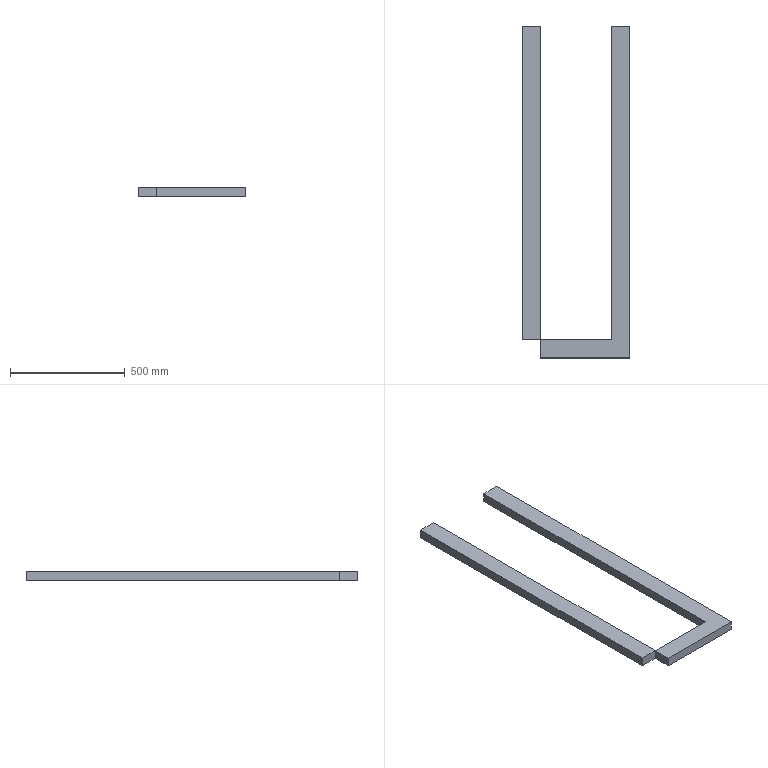Part | STEP file | Connecting profile | 2 solids | 14 faces | box 469.62 x 1446 x 40.945 mm | volume 10095669 mm3 | plane 14
STEP:
#1=CARTESIAN_POINT('',(0.,0.,0.));
#2=DIRECTION('',(0.,0.,1.));
#3=DIRECTION('',(1.,0.,0.));
#4=AXIS2_PLACEMENT_3D('',#1,#2,#3);
#5=CARTESIAN_POINT('',(0.,0.,0.));
#6=VERTEX_POINT('',#5);
#7=CARTESIAN_POINT('',(0.,-80.,0.));
#8=VERTEX_POINT('',#7);
#9=CARTESIAN_POINT('',(0.,-80.,0.));
#10=DIRECTION('',(0.,-1.,0.));
#11=VECTOR('',#10,1.);
#12=LINE('',#9,#11);
#13=CARTESIAN_POINT('',(0.,-80.,40.));
#14=DIRECTION('',(1.,0.,0.));
#15=DIRECTION('',(0.,0.,-1.));
#16=AXIS2_PLACEMENT_3D('',#13,#14,#15);
#17=PLANE('',#16);
#18=CARTESIAN_POINT('',(40.,0.));
#19=DIRECTION('',(0.,-1.));
#20=VECTOR('',#19,1.);
#21=LINE('',#18,#20);
#22=(GEOMETRIC_REPRESENTATION_CONTEXT(2)PARAMETRIC_REPRESENTATION_CONTEXT()REPRESENTATION_CONTEXT('',''));
#23=DEFINITIONAL_REPRESENTATION('',(#21),#22);
#24=PCURVE('',#17,#23);
#25=CARTESIAN_POINT('',(0.,0.,0.));
#26=DIRECTION('',(0.,0.,-1.));
#27=DIRECTION('',(-1.,0.,0.));
#28=AXIS2_PLACEMENT_3D('',#25,#26,#27);
#29=PLANE('',#28);
#30=CARTESIAN_POINT('',(0.,-80.));
#31=DIRECTION('',(0.,-1.));
#32=VECTOR('',#31,1.);
#33=LINE('',#30,#32);
#34=(GEOMETRIC_REPRESENTATION_CONTEXT(2)PARAMETRIC_REPRESENTATION_CONTEXT()REPRESENTATION_CONTEXT('',''));
#35=DEFINITIONAL_REPRESENTATION('',(#33),#34);
#36=PCURVE('',#29,#35);
#37=SURFACE_CURVE('',#12,(#24,#36),.PCURVE_S1.);
#38=EDGE_CURVE('',#6,#8,#37,.T.);
#39=ORIENTED_EDGE('',*,*,#38,.T.);
#40=CARTESIAN_POINT('',(0.,-80.,40.));
#41=VERTEX_POINT('',#40);
#42=CARTESIAN_POINT('',(0.,-80.,40.));
#43=DIRECTION('',(0.,0.,-1.));
#44=VECTOR('',#43,1.);
#45=LINE('',#42,#44);
#46=CARTESIAN_POINT('',(0.,0.));
#47=DIRECTION('',(1.,0.));
#48=VECTOR('',#47,1.);
#49=LINE('',#46,#48);
#50=(GEOMETRIC_REPRESENTATION_CONTEXT(2)PARAMETRIC_REPRESENTATION_CONTEXT()REPRESENTATION_CONTEXT('',''));
#51=DEFINITIONAL_REPRESENTATION('',(#49),#50);
#52=PCURVE('',#17,#51);
#53=CARTESIAN_POINT('',(389.62,-80.,40.));
#54=DIRECTION('',(0.,1.,0.));
#55=DIRECTION('',(-1.,0.,0.));
#56=AXIS2_PLACEMENT_3D('',#53,#54,#55);
#57=PLANE('',#56);
#58=CARTESIAN_POINT('',(389.62,0.));
#59=DIRECTION('',(0.,-1.));
#60=VECTOR('',#59,1.);
#61=LINE('',#58,#60);
#62=(GEOMETRIC_REPRESENTATION_CONTEXT(2)PARAMETRIC_REPRESENTATION_CONTEXT()REPRESENTATION_CONTEXT('',''));
#63=DEFINITIONAL_REPRESENTATION('',(#61),#62);
#64=PCURVE('',#57,#63);
#65=SURFACE_CURVE('',#45,(#52,#64),.PCURVE_S1.);
#66=EDGE_CURVE('',#41,#8,#65,.T.);
#67=ORIENTED_EDGE('',*,*,#66,.F.);
#68=CARTESIAN_POINT('',(0.,0.,40.));
#69=VERTEX_POINT('',#68);
#70=CARTESIAN_POINT('',(0.,-80.,40.));
#71=DIRECTION('',(0.,-1.,0.));
#72=VECTOR('',#71,1.);
#73=LINE('',#70,#72);
#74=CARTESIAN_POINT('',(0.,0.));
#75=DIRECTION('',(0.,-1.));
#76=VECTOR('',#75,1.);
#77=LINE('',#74,#76);
#78=(GEOMETRIC_REPRESENTATION_CONTEXT(2)PARAMETRIC_REPRESENTATION_CONTEXT()REPRESENTATION_CONTEXT('',''));
#79=DEFINITIONAL_REPRESENTATION('',(#77),#78);
#80=PCURVE('',#17,#79);
#81=CARTESIAN_POINT('',(0.,0.,40.));
#82=DIRECTION('',(0.,0.,-1.));
#83=DIRECTION('',(-1.,0.,0.));
#84=AXIS2_PLACEMENT_3D('',#81,#82,#83);
#85=PLANE('',#84);
#86=CARTESIAN_POINT('',(0.,-80.));
#87=DIRECTION('',(0.,-1.));
#88=VECTOR('',#87,1.);
#89=LINE('',#86,#88);
#90=(GEOMETRIC_REPRESENTATION_CONTEXT(2)PARAMETRIC_REPRESENTATION_CONTEXT()REPRESENTATION_CONTEXT('',''));
#91=DEFINITIONAL_REPRESENTATION('',(#89),#90);
#92=PCURVE('',#85,#91);
#93=SURFACE_CURVE('',#73,(#80,#92),.PCURVE_S1.);
#94=EDGE_CURVE('',#69,#41,#93,.T.);
#95=ORIENTED_EDGE('',*,*,#94,.F.);
#96=CARTESIAN_POINT('',(0.,0.,40.));
#97=DIRECTION('',(0.,0.,-1.));
#98=VECTOR('',#97,1.);
#99=LINE('',#96,#98);
#100=CARTESIAN_POINT('',(0.,80.));
#101=DIRECTION('',(1.,0.));
#102=VECTOR('',#101,1.);
#103=LINE('',#100,#102);
#104=(GEOMETRIC_REPRESENTATION_CONTEXT(2)PARAMETRIC_REPRESENTATION_CONTEXT()REPRESENTATION_CONTEXT('',''));
#105=DEFINITIONAL_REPRESENTATION('',(#103),#104);
#106=PCURVE('',#17,#105);
#107=CARTESIAN_POINT('',(0.,0.,40.));
#108=DIRECTION('',(0.,-1.,0.));
#109=DIRECTION('',(0.,0.,-1.));
#110=AXIS2_PLACEMENT_3D('',#107,#108,#109);
#111=PLANE('',#110);
#112=CARTESIAN_POINT('',(0.,0.));
#113=DIRECTION('',(1.,0.));
#114=VECTOR('',#113,1.);
#115=LINE('',#112,#114);
#116=(GEOMETRIC_REPRESENTATION_CONTEXT(2)PARAMETRIC_REPRESENTATION_CONTEXT()REPRESENTATION_CONTEXT('',''));
#117=DEFINITIONAL_REPRESENTATION('',(#115),#116);
#118=PCURVE('',#111,#117);
#119=SURFACE_CURVE('',#99,(#106,#118),.PCURVE_S1.);
#120=EDGE_CURVE('',#69,#6,#119,.T.);
#121=ORIENTED_EDGE('',*,*,#120,.T.);
#122=EDGE_LOOP('',(#39,#67,#95,#121));
#123=FACE_BOUND('',#122,.T.);
#124=ADVANCED_FACE('',(#123),#17,.F.);
#125=CARTESIAN_POINT('',(389.62,-80.,0.));
#126=VERTEX_POINT('',#125);
#127=CARTESIAN_POINT('',(389.62,-80.,0.));
#128=DIRECTION('',(1.,0.,0.));
#129=VECTOR('',#128,1.);
#130=LINE('',#127,#129);
#131=CARTESIAN_POINT('',(0.,-40.));
#132=DIRECTION('',(-1.,0.));
#133=VECTOR('',#132,1.);
#134=LINE('',#131,#133);
#135=(GEOMETRIC_REPRESENTATION_CONTEXT(2)PARAMETRIC_REPRESENTATION_CONTEXT()REPRESENTATION_CONTEXT('',''));
#136=DEFINITIONAL_REPRESENTATION('',(#134),#135);
#137=PCURVE('',#57,#136);
#138=CARTESIAN_POINT('',(-389.62,-80.));
#139=DIRECTION('',(-1.,0.));
#140=VECTOR('',#139,1.);
#141=LINE('',#138,#140);
#142=(GEOMETRIC_REPRESENTATION_CONTEXT(2)PARAMETRIC_REPRESENTATION_CONTEXT()REPRESENTATION_CONTEXT('',''));
#143=DEFINITIONAL_REPRESENTATION('',(#141),#142);
#144=PCURVE('',#29,#143);
#145=SURFACE_CURVE('',#130,(#137,#144),.PCURVE_S1.);
#146=EDGE_CURVE('',#8,#126,#145,.T.);
#147=ORIENTED_EDGE('',*,*,#146,.T.);
#148=CARTESIAN_POINT('',(389.62,-80.,40.));
#149=VERTEX_POINT('',#148);
#150=CARTESIAN_POINT('',(389.62,-80.,40.));
#151=DIRECTION('',(0.,0.,-1.));
#152=VECTOR('',#151,1.);
#153=LINE('',#150,#152);
#154=CARTESIAN_POINT('',(0.,0.));
#155=DIRECTION('',(0.,-1.));
#156=VECTOR('',#155,1.);
#157=LINE('',#154,#156);
#158=(GEOMETRIC_REPRESENTATION_CONTEXT(2)PARAMETRIC_REPRESENTATION_CONTEXT()REPRESENTATION_CONTEXT('',''));
#159=DEFINITIONAL_REPRESENTATION('',(#157),#158);
#160=PCURVE('',#57,#159);
#161=CARTESIAN_POINT('',(389.62,1366.5,40.));
#162=DIRECTION('',(-1.,0.,0.));
#163=DIRECTION('',(0.,-1.,0.));
#164=AXIS2_PLACEMENT_3D('',#161,#162,#163);
#165=PLANE('',#164);
#166=CARTESIAN_POINT('',(1446.5,0.));
#167=DIRECTION('',(0.,-1.));
#168=VECTOR('',#167,1.);
#169=LINE('',#166,#168);
#170=(GEOMETRIC_REPRESENTATION_CONTEXT(2)PARAMETRIC_REPRESENTATION_CONTEXT()REPRESENTATION_CONTEXT('',''));
#171=DEFINITIONAL_REPRESENTATION('',(#169),#170);
#172=PCURVE('',#165,#171);
#173=SURFACE_CURVE('',#153,(#160,#172),.PCURVE_S1.);
#174=EDGE_CURVE('',#149,#126,#173,.T.);
#175=ORIENTED_EDGE('',*,*,#174,.F.);
#176=CARTESIAN_POINT('',(389.62,-80.,40.));
#177=DIRECTION('',(1.,0.,0.));
#178=VECTOR('',#177,1.);
#179=LINE('',#176,#178);
#180=CARTESIAN_POINT('',(0.,0.));
#181=DIRECTION('',(-1.,0.));
#182=VECTOR('',#181,1.);
#183=LINE('',#180,#182);
#184=(GEOMETRIC_REPRESENTATION_CONTEXT(2)PARAMETRIC_REPRESENTATION_CONTEXT()REPRESENTATION_CONTEXT('',''));
#185=DEFINITIONAL_REPRESENTATION('',(#183),#184);
#186=PCURVE('',#57,#185);
#187=CARTESIAN_POINT('',(-389.62,-80.));
#188=DIRECTION('',(-1.,0.));
#189=VECTOR('',#188,1.);
#190=LINE('',#187,#189);
#191=(GEOMETRIC_REPRESENTATION_CONTEXT(2)PARAMETRIC_REPRESENTATION_CONTEXT()REPRESENTATION_CONTEXT('',''));
#192=DEFINITIONAL_REPRESENTATION('',(#190),#191);
#193=PCURVE('',#85,#192);
#194=SURFACE_CURVE('',#179,(#186,#193),.PCURVE_S1.);
#195=EDGE_CURVE('',#41,#149,#194,.T.);
#196=ORIENTED_EDGE('',*,*,#195,.F.);
#197=ORIENTED_EDGE('',*,*,#66,.T.);
#198=EDGE_LOOP('',(#147,#175,#196,#197));
#199=FACE_BOUND('',#198,.T.);
#200=ADVANCED_FACE('',(#199),#57,.F.);
#201=CARTESIAN_POINT('',(389.62,1366.5,0.));
#202=VERTEX_POINT('',#201);
#203=CARTESIAN_POINT('',(389.62,1366.5,0.));
#204=DIRECTION('',(0.,1.,0.));
#205=VECTOR('',#204,1.);
#206=LINE('',#203,#205);
#207=CARTESIAN_POINT('',(0.,-40.));
#208=DIRECTION('',(-1.,0.));
#209=VECTOR('',#208,1.);
#210=LINE('',#207,#209);
#211=(GEOMETRIC_REPRESENTATION_CONTEXT(2)PARAMETRIC_REPRESENTATION_CONTEXT()REPRESENTATION_CONTEXT('',''));
#212=DEFINITIONAL_REPRESENTATION('',(#210),#211);
#213=PCURVE('',#165,#212);
#214=CARTESIAN_POINT('',(-389.62,1366.5));
#215=DIRECTION('',(0.,1.));
#216=VECTOR('',#215,1.);
#217=LINE('',#214,#216);
#218=(GEOMETRIC_REPRESENTATION_CONTEXT(2)PARAMETRIC_REPRESENTATION_CONTEXT()REPRESENTATION_CONTEXT('',''));
#219=DEFINITIONAL_REPRESENTATION('',(#217),#218);
#220=PCURVE('',#29,#219);
#221=SURFACE_CURVE('',#206,(#213,#220),.PCURVE_S1.);
#222=EDGE_CURVE('',#126,#202,#221,.T.);
#223=ORIENTED_EDGE('',*,*,#222,.T.);
#224=CARTESIAN_POINT('',(389.62,1366.5,40.));
#225=VERTEX_POINT('',#224);
#226=CARTESIAN_POINT('',(389.62,1366.5,40.));
#227=DIRECTION('',(0.,0.,-1.));
#228=VECTOR('',#227,1.);
#229=LINE('',#226,#228);
#230=CARTESIAN_POINT('',(0.,0.));
#231=DIRECTION('',(0.,-1.));
#232=VECTOR('',#231,1.);
#233=LINE('',#230,#232);
#234=(GEOMETRIC_REPRESENTATION_CONTEXT(2)PARAMETRIC_REPRESENTATION_CONTEXT()REPRESENTATION_CONTEXT('',''));
#235=DEFINITIONAL_REPRESENTATION('',(#233),#234);
#236=PCURVE('',#165,#235);
#237=CARTESIAN_POINT('',(309.62,1366.5,40.));
#238=DIRECTION('',(0.,-1.,0.));
#239=DIRECTION('',(0.,0.,-1.));
#240=AXIS2_PLACEMENT_3D('',#237,#238,#239);
#241=PLANE('',#240);
#242=CARTESIAN_POINT('',(0.,80.));
#243=DIRECTION('',(1.,0.));
#244=VECTOR('',#243,1.);
#245=LINE('',#242,#244);
#246=(GEOMETRIC_REPRESENTATION_CONTEXT(2)PARAMETRIC_REPRESENTATION_CONTEXT()REPRESENTATION_CONTEXT('',''));
#247=DEFINITIONAL_REPRESENTATION('',(#245),#246);
#248=PCURVE('',#241,#247);
#249=SURFACE_CURVE('',#229,(#236,#248),.PCURVE_S1.);
#250=EDGE_CURVE('',#225,#202,#249,.T.);
#251=ORIENTED_EDGE('',*,*,#250,.F.);
#252=CARTESIAN_POINT('',(389.62,1366.5,40.));
#253=DIRECTION('',(0.,1.,0.));
#254=VECTOR('',#253,1.);
#255=LINE('',#252,#254);
#256=CARTESIAN_POINT('',(0.,0.));
#257=DIRECTION('',(-1.,0.));
#258=VECTOR('',#257,1.);
#259=LINE('',#256,#258);
#260=(GEOMETRIC_REPRESENTATION_CONTEXT(2)PARAMETRIC_REPRESENTATION_CONTEXT()REPRESENTATION_CONTEXT('',''));
#261=DEFINITIONAL_REPRESENTATION('',(#259),#260);
#262=PCURVE('',#165,#261);
#263=CARTESIAN_POINT('',(-389.62,1366.5));
#264=DIRECTION('',(0.,1.));
#265=VECTOR('',#264,1.);
#266=LINE('',#263,#265);
#267=(GEOMETRIC_REPRESENTATION_CONTEXT(2)PARAMETRIC_REPRESENTATION_CONTEXT()REPRESENTATION_CONTEXT('',''));
#268=DEFINITIONAL_REPRESENTATION('',(#266),#267);
#269=PCURVE('',#85,#268);
#270=SURFACE_CURVE('',#255,(#262,#269),.PCURVE_S1.);
#271=EDGE_CURVE('',#149,#225,#270,.T.);
#272=ORIENTED_EDGE('',*,*,#271,.F.);
#273=ORIENTED_EDGE('',*,*,#174,.T.);
#274=EDGE_LOOP('',(#223,#251,#272,#273));
#275=FACE_BOUND('',#274,.T.);
#276=ADVANCED_FACE('',(#275),#165,.F.);
#277=CARTESIAN_POINT('',(309.62,1366.5,0.));
#278=VERTEX_POINT('',#277);
#279=CARTESIAN_POINT('',(309.62,1366.5,0.));
#280=DIRECTION('',(-1.,0.,0.));
#281=VECTOR('',#280,1.);
#282=LINE('',#279,#281);
#283=CARTESIAN_POINT('',(40.,0.));
#284=DIRECTION('',(0.,-1.));
#285=VECTOR('',#284,1.);
#286=LINE('',#283,#285);
#287=(GEOMETRIC_REPRESENTATION_CONTEXT(2)PARAMETRIC_REPRESENTATION_CONTEXT()REPRESENTATION_CONTEXT('',''));
#288=DEFINITIONAL_REPRESENTATION('',(#286),#287);
#289=PCURVE('',#241,#288);
#290=CARTESIAN_POINT('',(-309.62,1366.5));
#291=DIRECTION('',(1.,0.));
#292=VECTOR('',#291,1.);
#293=LINE('',#290,#292);
#294=(GEOMETRIC_REPRESENTATION_CONTEXT(2)PARAMETRIC_REPRESENTATION_CONTEXT()REPRESENTATION_CONTEXT('',''));
#295=DEFINITIONAL_REPRESENTATION('',(#293),#294);
#296=PCURVE('',#29,#295);
#297=SURFACE_CURVE('',#282,(#289,#296),.PCURVE_S1.);
#298=EDGE_CURVE('',#202,#278,#297,.T.);
#299=ORIENTED_EDGE('',*,*,#298,.T.);
#300=CARTESIAN_POINT('',(309.62,1366.5,40.));
#301=VERTEX_POINT('',#300);
#302=CARTESIAN_POINT('',(309.62,1366.5,40.));
#303=DIRECTION('',(0.,0.,-1.));
#304=VECTOR('',#303,1.);
#305=LINE('',#302,#304);
#306=CARTESIAN_POINT('',(0.,0.));
#307=DIRECTION('',(1.,0.));
#308=VECTOR('',#307,1.);
#309=LINE('',#306,#308);
#310=(GEOMETRIC_REPRESENTATION_CONTEXT(2)PARAMETRIC_REPRESENTATION_CONTEXT()REPRESENTATION_CONTEXT('',''));
#311=DEFINITIONAL_REPRESENTATION('',(#309),#310);
#312=PCURVE('',#241,#311);
#313=CARTESIAN_POINT('',(309.62,0.,40.));
#314=DIRECTION('',(1.,0.,0.));
#315=DIRECTION('',(0.,0.,-1.));
#316=AXIS2_PLACEMENT_3D('',#313,#314,#315);
#317=PLANE('',#316);
#318=CARTESIAN_POINT('',(0.,1366.5));
#319=DIRECTION('',(1.,0.));
#320=VECTOR('',#319,1.);
#321=LINE('',#318,#320);
#322=(GEOMETRIC_REPRESENTATION_CONTEXT(2)PARAMETRIC_REPRESENTATION_CONTEXT()REPRESENTATION_CONTEXT('',''));
#323=DEFINITIONAL_REPRESENTATION('',(#321),#322);
#324=PCURVE('',#317,#323);
#325=SURFACE_CURVE('',#305,(#312,#324),.PCURVE_S1.);
#326=EDGE_CURVE('',#301,#278,#325,.T.);
#327=ORIENTED_EDGE('',*,*,#326,.F.);
#328=CARTESIAN_POINT('',(309.62,1366.5,40.));
#329=DIRECTION('',(-1.,0.,0.));
#330=VECTOR('',#329,1.);
#331=LINE('',#328,#330);
#332=CARTESIAN_POINT('',(0.,0.));
#333=DIRECTION('',(0.,-1.));
#334=VECTOR('',#333,1.);
#335=LINE('',#332,#334);
#336=(GEOMETRIC_REPRESENTATION_CONTEXT(2)PARAMETRIC_REPRESENTATION_CONTEXT()REPRESENTATION_CONTEXT('',''));
#337=DEFINITIONAL_REPRESENTATION('',(#335),#336);
#338=PCURVE('',#241,#337);
#339=CARTESIAN_POINT('',(-309.62,1366.5));
#340=DIRECTION('',(1.,0.));
#341=VECTOR('',#340,1.);
#342=LINE('',#339,#341);
#343=(GEOMETRIC_REPRESENTATION_CONTEXT(2)PARAMETRIC_REPRESENTATION_CONTEXT()REPRESENTATION_CONTEXT('',''));
#344=DEFINITIONAL_REPRESENTATION('',(#342),#343);
#345=PCURVE('',#85,#344);
#346=SURFACE_CURVE('',#331,(#338,#345),.PCURVE_S1.);
#347=EDGE_CURVE('',#225,#301,#346,.T.);
#348=ORIENTED_EDGE('',*,*,#347,.F.);
#349=ORIENTED_EDGE('',*,*,#250,.T.);
#350=EDGE_LOOP('',(#299,#327,#348,#349));
#351=FACE_BOUND('',#350,.T.);
#352=ADVANCED_FACE('',(#351),#241,.F.);
#353=CARTESIAN_POINT('',(309.62,0.,0.));
#354=VERTEX_POINT('',#353);
#355=CARTESIAN_POINT('',(309.62,0.,0.));
#356=DIRECTION('',(0.,-1.,0.));
#357=VECTOR('',#356,1.);
#358=LINE('',#355,#357);
#359=CARTESIAN_POINT('',(40.,0.));
#360=DIRECTION('',(0.,-1.));
#361=VECTOR('',#360,1.);
#362=LINE('',#359,#361);
#363=(GEOMETRIC_REPRESENTATION_CONTEXT(2)PARAMETRIC_REPRESENTATION_CONTEXT()REPRESENTATION_CONTEXT('',''));
#364=DEFINITIONAL_REPRESENTATION('',(#362),#363);
#365=PCURVE('',#317,#364);
#366=CARTESIAN_POINT('',(-309.62,0.));
#367=DIRECTION('',(0.,-1.));
#368=VECTOR('',#367,1.);
#369=LINE('',#366,#368);
#370=(GEOMETRIC_REPRESENTATION_CONTEXT(2)PARAMETRIC_REPRESENTATION_CONTEXT()REPRESENTATION_CONTEXT('',''));
#371=DEFINITIONAL_REPRESENTATION('',(#369),#370);
#372=PCURVE('',#29,#371);
#373=SURFACE_CURVE('',#358,(#365,#372),.PCURVE_S1.);
#374=EDGE_CURVE('',#278,#354,#373,.T.);
#375=ORIENTED_EDGE('',*,*,#374,.T.);
#376=CARTESIAN_POINT('',(309.62,0.,40.));
#377=VERTEX_POINT('',#376);
#378=CARTESIAN_POINT('',(309.62,0.,40.));
#379=DIRECTION('',(0.,0.,-1.));
#380=VECTOR('',#379,1.);
#381=LINE('',#378,#380);
#382=CARTESIAN_POINT('',(0.,0.));
#383=DIRECTION('',(1.,0.));
#384=VECTOR('',#383,1.);
#385=LINE('',#382,#384);
#386=(GEOMETRIC_REPRESENTATION_CONTEXT(2)PARAMETRIC_REPRESENTATION_CONTEXT()REPRESENTATION_CONTEXT('',''));
#387=DEFINITIONAL_REPRESENTATION('',(#385),#386);
#388=PCURVE('',#317,#387);
#389=CARTESIAN_POINT('',(0.,309.62));
#390=DIRECTION('',(1.,0.));
#391=VECTOR('',#390,1.);
#392=LINE('',#389,#391);
#393=(GEOMETRIC_REPRESENTATION_CONTEXT(2)PARAMETRIC_REPRESENTATION_CONTEXT()REPRESENTATION_CONTEXT('',''));
#394=DEFINITIONAL_REPRESENTATION('',(#392),#393);
#395=PCURVE('',#111,#394);
#396=SURFACE_CURVE('',#381,(#388,#395),.PCURVE_S1.);
#397=EDGE_CURVE('',#377,#354,#396,.T.);
#398=ORIENTED_EDGE('',*,*,#397,.F.);
#399=CARTESIAN_POINT('',(309.62,0.,40.));
#400=DIRECTION('',(0.,-1.,0.));
#401=VECTOR('',#400,1.);
#402=LINE('',#399,#401);
#403=CARTESIAN_POINT('',(0.,0.));
#404=DIRECTION('',(0.,-1.));
#405=VECTOR('',#404,1.);
#406=LINE('',#403,#405);
#407=(GEOMETRIC_REPRESENTATION_CONTEXT(2)PARAMETRIC_REPRESENTATION_CONTEXT()REPRESENTATION_CONTEXT('',''));
#408=DEFINITIONAL_REPRESENTATION('',(#406),#407);
#409=PCURVE('',#317,#408);
#410=CARTESIAN_POINT('',(-309.62,0.));
#411=DIRECTION('',(0.,-1.));
#412=VECTOR('',#411,1.);
#413=LINE('',#410,#412);
#414=(GEOMETRIC_REPRESENTATION_CONTEXT(2)PARAMETRIC_REPRESENTATION_CONTEXT()REPRESENTATION_CONTEXT('',''));
#415=DEFINITIONAL_REPRESENTATION('',(#413),#414);
#416=PCURVE('',#85,#415);
#417=SURFACE_CURVE('',#402,(#409,#416),.PCURVE_S1.);
#418=EDGE_CURVE('',#301,#377,#417,.T.);
#419=ORIENTED_EDGE('',*,*,#418,.F.);
#420=ORIENTED_EDGE('',*,*,#326,.T.);
#421=EDGE_LOOP('',(#375,#398,#419,#420));
#422=FACE_BOUND('',#421,.T.);
#423=ADVANCED_FACE('',(#422),#317,.F.);
#424=CARTESIAN_POINT('',(0.,0.,0.));
#425=DIRECTION('',(-1.,0.,0.));
#426=VECTOR('',#425,1.);
#427=LINE('',#424,#426);
#428=CARTESIAN_POINT('',(40.,0.));
#429=DIRECTION('',(0.,-1.));
#430=VECTOR('',#429,1.);
#431=LINE('',#428,#430);
#432=(GEOMETRIC_REPRESENTATION_CONTEXT(2)PARAMETRIC_REPRESENTATION_CONTEXT()REPRESENTATION_CONTEXT('',''));
#433=DEFINITIONAL_REPRESENTATION('',(#431),#432);
#434=PCURVE('',#111,#433);
#435=CARTESIAN_POINT('',(0.,0.));
#436=DIRECTION('',(1.,0.));
#437=VECTOR('',#436,1.);
#438=LINE('',#435,#437);
#439=(GEOMETRIC_REPRESENTATION_CONTEXT(2)PARAMETRIC_REPRESENTATION_CONTEXT()REPRESENTATION_CONTEXT('',''));
#440=DEFINITIONAL_REPRESENTATION('',(#438),#439);
#441=PCURVE('',#29,#440);
#442=SURFACE_CURVE('',#427,(#434,#441),.PCURVE_S1.);
#443=EDGE_CURVE('',#354,#6,#442,.T.);
#444=ORIENTED_EDGE('',*,*,#443,.T.);
#445=ORIENTED_EDGE('',*,*,#120,.F.);
#446=CARTESIAN_POINT('',(0.,0.,40.));
#447=DIRECTION('',(-1.,0.,0.));
#448=VECTOR('',#447,1.);
#449=LINE('',#446,#448);
#450=CARTESIAN_POINT('',(0.,0.));
#451=DIRECTION('',(0.,-1.));
#452=VECTOR('',#451,1.);
#453=LINE('',#450,#452);
#454=(GEOMETRIC_REPRESENTATION_CONTEXT(2)PARAMETRIC_REPRESENTATION_CONTEXT()REPRESENTATION_CONTEXT('',''));
#455=DEFINITIONAL_REPRESENTATION('',(#453),#454);
#456=PCURVE('',#111,#455);
#457=CARTESIAN_POINT('',(0.,0.));
#458=DIRECTION('',(1.,0.));
#459=VECTOR('',#458,1.);
#460=LINE('',#457,#459);
#461=(GEOMETRIC_REPRESENTATION_CONTEXT(2)PARAMETRIC_REPRESENTATION_CONTEXT()REPRESENTATION_CONTEXT('',''));
#462=DEFINITIONAL_REPRESENTATION('',(#460),#461);
#463=PCURVE('',#85,#462);
#464=SURFACE_CURVE('',#449,(#456,#463),.PCURVE_S1.);
#465=EDGE_CURVE('',#377,#69,#464,.T.);
#466=ORIENTED_EDGE('',*,*,#465,.F.);
#467=ORIENTED_EDGE('',*,*,#397,.T.);
#468=EDGE_LOOP('',(#444,#445,#466,#467));
#469=FACE_BOUND('',#468,.T.);
#470=ADVANCED_FACE('',(#469),#111,.F.);
#471=ORIENTED_EDGE('',*,*,#94,.T.);
#472=ORIENTED_EDGE('',*,*,#195,.T.);
#473=ORIENTED_EDGE('',*,*,#271,.T.);
#474=ORIENTED_EDGE('',*,*,#347,.T.);
#475=ORIENTED_EDGE('',*,*,#418,.T.);
#476=ORIENTED_EDGE('',*,*,#465,.T.);
#477=EDGE_LOOP('',(#471,#472,#473,#474,#475,#476));
#478=FACE_BOUND('',#477,.T.);
#479=ADVANCED_FACE('',(#478),#85,.F.);
#480=ORIENTED_EDGE('',*,*,#38,.F.);
#481=ORIENTED_EDGE('',*,*,#443,.F.);
#482=ORIENTED_EDGE('',*,*,#374,.F.);
#483=ORIENTED_EDGE('',*,*,#298,.F.);
#484=ORIENTED_EDGE('',*,*,#222,.F.);
#485=ORIENTED_EDGE('',*,*,#146,.F.);
#486=EDGE_LOOP('',(#480,#481,#482,#483,#484,#485));
#487=FACE_BOUND('',#486,.T.);
#488=ADVANCED_FACE('',(#487),#29,.T.);
#489=CLOSED_SHELL('',(#124,#200,#276,#352,#423,#470,#479,#488));
#490=MANIFOLD_SOLID_BREP('',#489);
#491=CARTESIAN_POINT('',(0.,0.,40.945));
#492=VERTEX_POINT('',#491);
#493=CARTESIAN_POINT('',(0.,0.,0.));
#494=VERTEX_POINT('',#493);
#495=CARTESIAN_POINT('',(0.,0.,0.));
#496=DIRECTION('',(0.,0.,-1.));
#497=VECTOR('',#496,1.);
#498=LINE('',#495,#497);
#499=CARTESIAN_POINT('',(0.,0.,40.945));
#500=DIRECTION('',(0.,-1.,0.));
#501=DIRECTION('',(0.,0.,-1.));
#502=AXIS2_PLACEMENT_3D('',#499,#500,#501);
#503=PLANE('',#502);
#504=CARTESIAN_POINT('',(40.945,0.));
#505=DIRECTION('',(1.,0.));
#506=VECTOR('',#505,1.);
#507=LINE('',#504,#506);
#508=(GEOMETRIC_REPRESENTATION_CONTEXT(2)PARAMETRIC_REPRESENTATION_CONTEXT()REPRESENTATION_CONTEXT('',''));
#509=DEFINITIONAL_REPRESENTATION('',(#507),#508);
#510=PCURVE('',#503,#509);
#511=CARTESIAN_POINT('',(0.,1456.369,0.));
#512=DIRECTION('',(-1.,0.,0.));
#513=DIRECTION('',(0.,0.,1.));
#514=AXIS2_PLACEMENT_3D('',#511,#512,#513);
#515=PLANE('',#514);
#516=CARTESIAN_POINT('',(0.,-1456.369));
#517=DIRECTION('',(-1.,0.));
#518=VECTOR('',#517,1.);
#519=LINE('',#516,#518);
#520=(GEOMETRIC_REPRESENTATION_CONTEXT(2)PARAMETRIC_REPRESENTATION_CONTEXT()REPRESENTATION_CONTEXT('',''));
#521=DEFINITIONAL_REPRESENTATION('',(#519),#520);
#522=PCURVE('',#515,#521);
#523=SURFACE_CURVE('',#498,(#510,#522),.PCURVE_S1.);
#524=EDGE_CURVE('',#492,#494,#523,.T.);
#525=ORIENTED_EDGE('',*,*,#524,.F.);
#526=CARTESIAN_POINT('',(-80.,0.,40.945));
#527=VERTEX_POINT('',#526);
#528=CARTESIAN_POINT('',(0.,0.,40.945));
#529=DIRECTION('',(1.,0.,0.));
#530=VECTOR('',#529,1.);
#531=LINE('',#528,#530);
#532=CARTESIAN_POINT('',(0.,0.));
#533=DIRECTION('',(0.,1.));
#534=VECTOR('',#533,1.);
#535=LINE('',#532,#534);
#536=(GEOMETRIC_REPRESENTATION_CONTEXT(2)PARAMETRIC_REPRESENTATION_CONTEXT()REPRESENTATION_CONTEXT('',''));
#537=DEFINITIONAL_REPRESENTATION('',(#535),#536);
#538=PCURVE('',#503,#537);
#539=CARTESIAN_POINT('',(0.,1456.369,40.945));
#540=DIRECTION('',(0.,0.,-1.));
#541=DIRECTION('',(-1.,0.,0.));
#542=AXIS2_PLACEMENT_3D('',#539,#540,#541);
#543=PLANE('',#542);
#544=CARTESIAN_POINT('',(0.,-1456.369));
#545=DIRECTION('',(-1.,0.));
#546=VECTOR('',#545,1.);
#547=LINE('',#544,#546);
#548=(GEOMETRIC_REPRESENTATION_CONTEXT(2)PARAMETRIC_REPRESENTATION_CONTEXT()REPRESENTATION_CONTEXT('',''));
#549=DEFINITIONAL_REPRESENTATION('',(#547),#548);
#550=PCURVE('',#543,#549);
#551=SURFACE_CURVE('',#531,(#538,#550),.PCURVE_S1.);
#552=EDGE_CURVE('',#527,#492,#551,.T.);
#553=ORIENTED_EDGE('',*,*,#552,.F.);
#554=CARTESIAN_POINT('',(-80.,0.,0.));
#555=VERTEX_POINT('',#554);
#556=CARTESIAN_POINT('',(-80.,0.,0.));
#557=DIRECTION('',(0.,0.,1.));
#558=VECTOR('',#557,1.);
#559=LINE('',#556,#558);
#560=CARTESIAN_POINT('',(40.945,-80.));
#561=DIRECTION('',(-1.,0.));
#562=VECTOR('',#561,1.);
#563=LINE('',#560,#562);
#564=(GEOMETRIC_REPRESENTATION_CONTEXT(2)PARAMETRIC_REPRESENTATION_CONTEXT()REPRESENTATION_CONTEXT('',''));
#565=DEFINITIONAL_REPRESENTATION('',(#563),#564);
#566=PCURVE('',#503,#565);
#567=CARTESIAN_POINT('',(-80.,1456.369,0.));
#568=DIRECTION('',(1.,0.,0.));
#569=DIRECTION('',(0.,0.,-1.));
#570=AXIS2_PLACEMENT_3D('',#567,#568,#569);
#571=PLANE('',#570);
#572=CARTESIAN_POINT('',(0.,-1456.369));
#573=DIRECTION('',(-1.,0.));
#574=VECTOR('',#573,1.);
#575=LINE('',#572,#574);
#576=(GEOMETRIC_REPRESENTATION_CONTEXT(2)PARAMETRIC_REPRESENTATION_CONTEXT()REPRESENTATION_CONTEXT('',''));
#577=DEFINITIONAL_REPRESENTATION('',(#575),#576);
#578=PCURVE('',#571,#577);
#579=SURFACE_CURVE('',#559,(#566,#578),.PCURVE_S1.);
#580=EDGE_CURVE('',#555,#527,#579,.T.);
#581=ORIENTED_EDGE('',*,*,#580,.F.);
#582=CARTESIAN_POINT('',(0.,0.,0.));
#583=DIRECTION('',(-1.,0.,0.));
#584=VECTOR('',#583,1.);
#585=LINE('',#582,#584);
#586=CARTESIAN_POINT('',(40.945,0.));
#587=DIRECTION('',(0.,-1.));
#588=VECTOR('',#587,1.);
#589=LINE('',#586,#588);
#590=(GEOMETRIC_REPRESENTATION_CONTEXT(2)PARAMETRIC_REPRESENTATION_CONTEXT()REPRESENTATION_CONTEXT('',''));
#591=DEFINITIONAL_REPRESENTATION('',(#589),#590);
#592=PCURVE('',#503,#591);
#593=CARTESIAN_POINT('',(0.,1456.369,0.));
#594=DIRECTION('',(0.,0.,1.));
#595=DIRECTION('',(1.,0.,0.));
#596=AXIS2_PLACEMENT_3D('',#593,#594,#595);
#597=PLANE('',#596);
#598=CARTESIAN_POINT('',(0.,-1456.369));
#599=DIRECTION('',(-1.,0.));
#600=VECTOR('',#599,1.);
#601=LINE('',#598,#600);
#602=(GEOMETRIC_REPRESENTATION_CONTEXT(2)PARAMETRIC_REPRESENTATION_CONTEXT()REPRESENTATION_CONTEXT('',''));
#603=DEFINITIONAL_REPRESENTATION('',(#601),#602);
#604=PCURVE('',#597,#603);
#605=SURFACE_CURVE('',#585,(#592,#604),.PCURVE_S1.);
#606=EDGE_CURVE('',#494,#555,#605,.T.);
#607=ORIENTED_EDGE('',*,*,#606,.F.);
#608=EDGE_LOOP('',(#525,#553,#581,#607));
#609=FACE_BOUND('',#608,.T.);
#610=ADVANCED_FACE('',(#609),#503,.T.);
#611=CARTESIAN_POINT('',(0.,1366.5,40.945));
#612=VERTEX_POINT('',#611);
#613=CARTESIAN_POINT('',(0.,1456.369,40.945));
#614=DIRECTION('',(0.,-1.,0.));
#615=VECTOR('',#614,1.);
#616=LINE('',#613,#615);
#617=CARTESIAN_POINT('',(0.,0.));
#618=DIRECTION('',(0.,-1.));
#619=VECTOR('',#618,1.);
#620=LINE('',#617,#619);
#621=(GEOMETRIC_REPRESENTATION_CONTEXT(2)PARAMETRIC_REPRESENTATION_CONTEXT()REPRESENTATION_CONTEXT('',''));
#622=DEFINITIONAL_REPRESENTATION('',(#620),#621);
#623=PCURVE('',#543,#622);
#624=CARTESIAN_POINT('',(40.945,0.));
#625=DIRECTION('',(0.,-1.));
#626=VECTOR('',#625,1.);
#627=LINE('',#624,#626);
#628=(GEOMETRIC_REPRESENTATION_CONTEXT(2)PARAMETRIC_REPRESENTATION_CONTEXT()REPRESENTATION_CONTEXT('',''));
#629=DEFINITIONAL_REPRESENTATION('',(#627),#628);
#630=PCURVE('',#515,#629);
#631=SURFACE_CURVE('',#616,(#623,#630),.PCURVE_S1.);
#632=EDGE_CURVE('',#612,#492,#631,.T.);
#633=ORIENTED_EDGE('',*,*,#632,.F.);
#634=CARTESIAN_POINT('',(-80.,1366.5,40.945));
#635=VERTEX_POINT('',#634);
#636=CARTESIAN_POINT('',(0.,1366.5,40.945));
#637=DIRECTION('',(-1.,0.,0.));
#638=VECTOR('',#637,1.);
#639=LINE('',#636,#638);
#640=CARTESIAN_POINT('',(0.,-89.869));
#641=DIRECTION('',(1.,0.));
#642=VECTOR('',#641,1.);
#643=LINE('',#640,#642);
#644=(GEOMETRIC_REPRESENTATION_CONTEXT(2)PARAMETRIC_REPRESENTATION_CONTEXT()REPRESENTATION_CONTEXT('',''));
#645=DEFINITIONAL_REPRESENTATION('',(#643),#644);
#646=PCURVE('',#543,#645);
#647=CARTESIAN_POINT('',(309.62,1366.5,40.));
#648=DIRECTION('',(0.,-1.,0.));
#649=DIRECTION('',(0.,0.,-1.));
#650=AXIS2_PLACEMENT_3D('',#647,#648,#649);
#651=PLANE('',#650);
#652=CARTESIAN_POINT('',(-0.9448,-309.62));
#653=DIRECTION('',(0.,-1.));
#654=VECTOR('',#653,1.);
#655=LINE('',#652,#654);
#656=(GEOMETRIC_REPRESENTATION_CONTEXT(2)PARAMETRIC_REPRESENTATION_CONTEXT()REPRESENTATION_CONTEXT('',''));
#657=DEFINITIONAL_REPRESENTATION('',(#655),#656);
#658=PCURVE('',#651,#657);
#659=SURFACE_CURVE('',#639,(#646,#658),.PCURVE_S1.);
#660=EDGE_CURVE('',#612,#635,#659,.T.);
#661=ORIENTED_EDGE('',*,*,#660,.T.);
#662=CARTESIAN_POINT('',(-80.,1456.369,40.945));
#663=DIRECTION('',(0.,-1.,0.));
#664=VECTOR('',#663,1.);
#665=LINE('',#662,#664);
#666=CARTESIAN_POINT('',(80.,0.));
#667=DIRECTION('',(0.,-1.));
#668=VECTOR('',#667,1.);
#669=LINE('',#666,#668);
#670=(GEOMETRIC_REPRESENTATION_CONTEXT(2)PARAMETRIC_REPRESENTATION_CONTEXT()REPRESENTATION_CONTEXT('',''));
#671=DEFINITIONAL_REPRESENTATION('',(#669),#670);
#672=PCURVE('',#543,#671);
#673=CARTESIAN_POINT('',(-40.945,0.));
#674=DIRECTION('',(0.,-1.));
#675=VECTOR('',#674,1.);
#676=LINE('',#673,#675);
#677=(GEOMETRIC_REPRESENTATION_CONTEXT(2)PARAMETRIC_REPRESENTATION_CONTEXT()REPRESENTATION_CONTEXT('',''));
#678=DEFINITIONAL_REPRESENTATION('',(#676),#677);
#679=PCURVE('',#571,#678);
#680=SURFACE_CURVE('',#665,(#672,#679),.PCURVE_S1.);
#681=EDGE_CURVE('',#635,#527,#680,.T.);
#682=ORIENTED_EDGE('',*,*,#681,.T.);
#683=ORIENTED_EDGE('',*,*,#552,.T.);
#684=EDGE_LOOP('',(#633,#661,#682,#683));
#685=FACE_BOUND('',#684,.T.);
#686=ADVANCED_FACE('',(#685),#543,.F.);
#687=ORIENTED_EDGE('',*,*,#681,.F.);
#688=CARTESIAN_POINT('',(-80.,1366.5,0.));
#689=VERTEX_POINT('',#688);
#690=CARTESIAN_POINT('',(-80.,1366.5,0.));
#691=DIRECTION('',(0.,0.,-1.));
#692=VECTOR('',#691,1.);
#693=LINE('',#690,#692);
#694=CARTESIAN_POINT('',(0.,-89.869));
#695=DIRECTION('',(1.,0.));
#696=VECTOR('',#695,1.);
#697=LINE('',#694,#696);
#698=(GEOMETRIC_REPRESENTATION_CONTEXT(2)PARAMETRIC_REPRESENTATION_CONTEXT()REPRESENTATION_CONTEXT('',''));
#699=DEFINITIONAL_REPRESENTATION('',(#697),#698);
#700=PCURVE('',#571,#699);
#701=CARTESIAN_POINT('',(40.,-389.62));
#702=DIRECTION('',(1.,0.));
#703=VECTOR('',#702,1.);
#704=LINE('',#701,#703);
#705=(GEOMETRIC_REPRESENTATION_CONTEXT(2)PARAMETRIC_REPRESENTATION_CONTEXT()REPRESENTATION_CONTEXT('',''));
#706=DEFINITIONAL_REPRESENTATION('',(#704),#705);
#707=PCURVE('',#651,#706);
#708=SURFACE_CURVE('',#693,(#700,#707),.PCURVE_S1.);
#709=EDGE_CURVE('',#635,#689,#708,.T.);
#710=ORIENTED_EDGE('',*,*,#709,.T.);
#711=CARTESIAN_POINT('',(-80.,1456.369,0.));
#712=DIRECTION('',(0.,-1.,0.));
#713=VECTOR('',#712,1.);
#714=LINE('',#711,#713);
#715=CARTESIAN_POINT('',(0.,0.));
#716=DIRECTION('',(0.,-1.));
#717=VECTOR('',#716,1.);
#718=LINE('',#715,#717);
#719=(GEOMETRIC_REPRESENTATION_CONTEXT(2)PARAMETRIC_REPRESENTATION_CONTEXT()REPRESENTATION_CONTEXT('',''));
#720=DEFINITIONAL_REPRESENTATION('',(#718),#719);
#721=PCURVE('',#571,#720);
#722=CARTESIAN_POINT('',(-80.,0.));
#723=DIRECTION('',(0.,-1.));
#724=VECTOR('',#723,1.);
#725=LINE('',#722,#724);
#726=(GEOMETRIC_REPRESENTATION_CONTEXT(2)PARAMETRIC_REPRESENTATION_CONTEXT()REPRESENTATION_CONTEXT('',''));
#727=DEFINITIONAL_REPRESENTATION('',(#725),#726);
#728=PCURVE('',#597,#727);
#729=SURFACE_CURVE('',#714,(#721,#728),.PCURVE_S1.);
#730=EDGE_CURVE('',#689,#555,#729,.T.);
#731=ORIENTED_EDGE('',*,*,#730,.T.);
#732=ORIENTED_EDGE('',*,*,#580,.T.);
#733=EDGE_LOOP('',(#687,#710,#731,#732));
#734=FACE_BOUND('',#733,.T.);
#735=ADVANCED_FACE('',(#734),#571,.F.);
#736=ORIENTED_EDGE('',*,*,#730,.F.);
#737=CARTESIAN_POINT('',(0.,1366.5,0.));
#738=VERTEX_POINT('',#737);
#739=CARTESIAN_POINT('',(0.,1366.5,0.));
#740=DIRECTION('',(1.,0.,0.));
#741=VECTOR('',#740,1.);
#742=LINE('',#739,#741);
#743=CARTESIAN_POINT('',(0.,-89.869));
#744=DIRECTION('',(1.,0.));
#745=VECTOR('',#744,1.);
#746=LINE('',#743,#745);
#747=(GEOMETRIC_REPRESENTATION_CONTEXT(2)PARAMETRIC_REPRESENTATION_CONTEXT()REPRESENTATION_CONTEXT('',''));
#748=DEFINITIONAL_REPRESENTATION('',(#746),#747);
#749=PCURVE('',#597,#748);
#750=CARTESIAN_POINT('',(40.,-309.62));
#751=DIRECTION('',(0.,1.));
#752=VECTOR('',#751,1.);
#753=LINE('',#750,#752);
#754=(GEOMETRIC_REPRESENTATION_CONTEXT(2)PARAMETRIC_REPRESENTATION_CONTEXT()REPRESENTATION_CONTEXT('',''));
#755=DEFINITIONAL_REPRESENTATION('',(#753),#754);
#756=PCURVE('',#651,#755);
#757=SURFACE_CURVE('',#742,(#749,#756),.PCURVE_S1.);
#758=EDGE_CURVE('',#689,#738,#757,.T.);
#759=ORIENTED_EDGE('',*,*,#758,.T.);
#760=CARTESIAN_POINT('',(0.,1456.369,0.));
#761=DIRECTION('',(0.,-1.,0.));
#762=VECTOR('',#761,1.);
#763=LINE('',#760,#762);
#764=CARTESIAN_POINT('',(0.,0.));
#765=DIRECTION('',(0.,-1.));
#766=VECTOR('',#765,1.);
#767=LINE('',#764,#766);
#768=(GEOMETRIC_REPRESENTATION_CONTEXT(2)PARAMETRIC_REPRESENTATION_CONTEXT()REPRESENTATION_CONTEXT('',''));
#769=DEFINITIONAL_REPRESENTATION('',(#767),#768);
#770=PCURVE('',#597,#769);
#771=CARTESIAN_POINT('',(0.,0.));
#772=DIRECTION('',(0.,-1.));
#773=VECTOR('',#772,1.);
#774=LINE('',#771,#773);
#775=(GEOMETRIC_REPRESENTATION_CONTEXT(2)PARAMETRIC_REPRESENTATION_CONTEXT()REPRESENTATION_CONTEXT('',''));
#776=DEFINITIONAL_REPRESENTATION('',(#774),#775);
#777=PCURVE('',#515,#776);
#778=SURFACE_CURVE('',#763,(#770,#777),.PCURVE_S1.);
#779=EDGE_CURVE('',#738,#494,#778,.T.);
#780=ORIENTED_EDGE('',*,*,#779,.T.);
#781=ORIENTED_EDGE('',*,*,#606,.T.);
#782=EDGE_LOOP('',(#736,#759,#780,#781));
#783=FACE_BOUND('',#782,.T.);
#784=ADVANCED_FACE('',(#783),#597,.F.);
#785=ORIENTED_EDGE('',*,*,#779,.F.);
#786=CARTESIAN_POINT('',(0.,1366.5,0.));
#787=DIRECTION('',(0.,0.,1.));
#788=VECTOR('',#787,1.);
#789=LINE('',#786,#788);
#790=CARTESIAN_POINT('',(0.,-89.869));
#791=DIRECTION('',(1.,0.));
#792=VECTOR('',#791,1.);
#793=LINE('',#790,#792);
#794=(GEOMETRIC_REPRESENTATION_CONTEXT(2)PARAMETRIC_REPRESENTATION_CONTEXT()REPRESENTATION_CONTEXT('',''));
#795=DEFINITIONAL_REPRESENTATION('',(#793),#794);
#796=PCURVE('',#515,#795);
#797=CARTESIAN_POINT('',(40.,-309.62));
#798=DIRECTION('',(-1.,0.));
#799=VECTOR('',#798,1.);
#800=LINE('',#797,#799);
#801=(GEOMETRIC_REPRESENTATION_CONTEXT(2)PARAMETRIC_REPRESENTATION_CONTEXT()REPRESENTATION_CONTEXT('',''));
#802=DEFINITIONAL_REPRESENTATION('',(#800),#801);
#803=PCURVE('',#651,#802);
#804=SURFACE_CURVE('',#789,(#796,#803),.PCURVE_S1.);
#805=EDGE_CURVE('',#738,#612,#804,.T.);
#806=ORIENTED_EDGE('',*,*,#805,.T.);
#807=ORIENTED_EDGE('',*,*,#632,.T.);
#808=ORIENTED_EDGE('',*,*,#524,.T.);
#809=EDGE_LOOP('',(#785,#806,#807,#808));
#810=FACE_BOUND('',#809,.T.);
#811=ADVANCED_FACE('',(#810),#515,.F.);
#812=ORIENTED_EDGE('',*,*,#758,.F.);
#813=ORIENTED_EDGE('',*,*,#709,.F.);
#814=ORIENTED_EDGE('',*,*,#660,.F.);
#815=ORIENTED_EDGE('',*,*,#805,.F.);
#816=EDGE_LOOP('',(#812,#813,#814,#815));
#817=FACE_BOUND('',#816,.T.);
#818=ADVANCED_FACE('',(#817),#651,.F.);
#819=CLOSED_SHELL('',(#610,#686,#735,#784,#811,#818));
#820=MANIFOLD_SOLID_BREP('',#819);
#821=(LENGTH_UNIT()NAMED_UNIT(*)SI_UNIT(.MILLI.,.METRE.));
#822=UNCERTAINTY_MEASURE_WITH_UNIT(LENGTH_MEASURE(0.0000001),#821,'','');
#823=(NAMED_UNIT(*)PLANE_ANGLE_UNIT()SI_UNIT($,.RADIAN.));
#824=(NAMED_UNIT(*)SI_UNIT($,.STERADIAN.)SOLID_ANGLE_UNIT());
#825=(GEOMETRIC_REPRESENTATION_CONTEXT(3)GLOBAL_UNCERTAINTY_ASSIGNED_CONTEXT((#822))GLOBAL_UNIT_ASSIGNED_CONTEXT((#821,#823,#824))REPRESENTATION_CONTEXT('',''));
#826=SHAPE_REPRESENTATION('',(#4,#490,#820),#825);